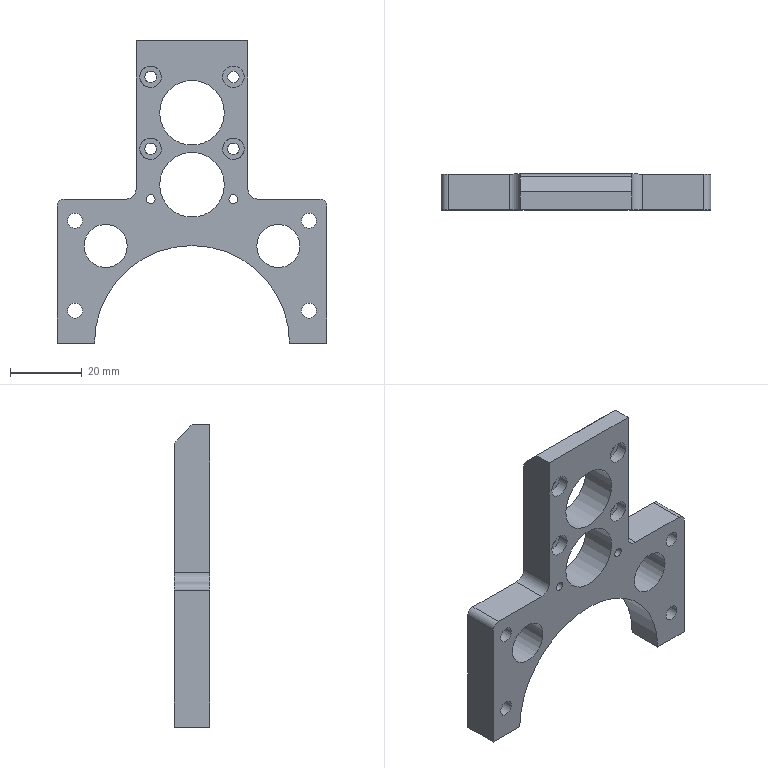Part | NX | 1 solid | 40 faces | box 75 x 10 x 84 mm | volume 23164 mm3 | cylinder 24 | plane 16 | commonest cylinder face diameters 6 x7 3.2 x4 4.2 x4 2.5 x2 4 x2 12 x2
STEP:
#1=CARTESIAN_POINT('',(-15.5,-5.,42.));
#2=VERTEX_POINT('',#1);
#3=CARTESIAN_POINT('',(-15.5,0.,42.));
#4=VERTEX_POINT('',#3);
#5=CARTESIAN_POINT('',(-15.5,-5.,42.));
#6=DIRECTION('',(0.,1.,0.));
#7=VECTOR('',#6,1000.);
#8=LINE('',#5,#7);
#9=EDGE_CURVE('',#2,#4,#8,.T.);
#10=ORIENTED_EDGE('',*,*,#9,.F.);
#11=CARTESIAN_POINT('',(15.5,-5.,42.));
#12=VERTEX_POINT('',#11);
#13=CARTESIAN_POINT('',(-15.5,-5.,42.));
#14=DIRECTION('',(1.,0.,0.));
#15=VECTOR('',#14,1000.);
#16=LINE('',#13,#15);
#17=EDGE_CURVE('',#2,#12,#16,.T.);
#18=ORIENTED_EDGE('',*,*,#17,.T.);
#19=CARTESIAN_POINT('',(15.5,0.,42.));
#20=VERTEX_POINT('',#19);
#21=CARTESIAN_POINT('',(15.5,-5.,42.));
#22=DIRECTION('',(0.,1.,0.));
#23=VECTOR('',#22,1000.);
#24=LINE('',#21,#23);
#25=EDGE_CURVE('',#12,#20,#24,.T.);
#26=ORIENTED_EDGE('',*,*,#25,.T.);
#27=CARTESIAN_POINT('',(-15.5,0.,42.));
#28=DIRECTION('',(1.,0.,0.));
#29=VECTOR('',#28,1000.);
#30=LINE('',#27,#29);
#31=EDGE_CURVE('',#4,#20,#30,.T.);
#32=ORIENTED_EDGE('',*,*,#31,.F.);
#33=EDGE_LOOP('',(#10,#18,#26,#32));
#34=FACE_BOUND('',#33,.T.);
#35=CARTESIAN_POINT('',(-37.5,-5.,42.));
#36=DIRECTION('',(0.,0.,1.));
#37=DIRECTION('',(1.,0.,0.));
#38=AXIS2_PLACEMENT_3D('',#35,#36,#37);
#39=PLANE('',#38);
#40=ADVANCED_FACE('',(#34),#39,.T.);
#41=CARTESIAN_POINT('',(-15.5,4.121,37.879));
#42=VERTEX_POINT('',#41);
#43=CARTESIAN_POINT('',(-15.5,0.,42.));
#44=DIRECTION('',(0.,0.7071,-0.7071));
#45=VECTOR('',#44,1000.);
#46=LINE('',#43,#45);
#47=EDGE_CURVE('',#4,#42,#46,.T.);
#48=ORIENTED_EDGE('',*,*,#47,.F.);
#49=ORIENTED_EDGE('',*,*,#31,.T.);
#50=CARTESIAN_POINT('',(15.5,4.121,37.879));
#51=VERTEX_POINT('',#50);
#52=CARTESIAN_POINT('',(15.5,4.121,37.879));
#53=DIRECTION('',(0.,-0.7071,0.7071));
#54=VECTOR('',#53,1000.);
#55=LINE('',#52,#54);
#56=EDGE_CURVE('',#51,#20,#55,.T.);
#57=ORIENTED_EDGE('',*,*,#56,.F.);
#58=CARTESIAN_POINT('',(-15.5,4.121,37.879));
#59=DIRECTION('',(1.,0.,0.));
#60=VECTOR('',#59,1000.);
#61=LINE('',#58,#60);
#62=EDGE_CURVE('',#42,#51,#61,.T.);
#63=ORIENTED_EDGE('',*,*,#62,.F.);
#64=EDGE_LOOP('',(#48,#49,#57,#63));
#65=FACE_BOUND('',#64,.T.);
#66=CARTESIAN_POINT('',(0.,2.5,39.5));
#67=DIRECTION('',(0.,0.7071,0.7071));
#68=DIRECTION('',(0.,-0.7071,0.7071));
#69=AXIS2_PLACEMENT_3D('',#66,#67,#68);
#70=PLANE('',#69);
#71=ADVANCED_FACE('',(#65),#70,.T.);
#72=CARTESIAN_POINT('',(-15.5,5.,35.757));
#73=VERTEX_POINT('',#72);
#74=CARTESIAN_POINT('',(-15.5,5.,1.));
#75=VERTEX_POINT('',#74);
#76=CARTESIAN_POINT('',(-15.5,5.,35.757));
#77=DIRECTION('',(0.,0.,-1.));
#78=VECTOR('',#77,1000.);
#79=LINE('',#76,#78);
#80=EDGE_CURVE('',#73,#75,#79,.T.);
#81=ORIENTED_EDGE('',*,*,#80,.T.);
#82=CARTESIAN_POINT('',(-15.5,-5.,1.));
#83=VERTEX_POINT('',#82);
#84=CARTESIAN_POINT('',(-15.5,5.,1.));
#85=DIRECTION('',(0.,-1.,0.));
#86=VECTOR('',#85,1000.);
#87=LINE('',#84,#86);
#88=EDGE_CURVE('',#75,#83,#87,.T.);
#89=ORIENTED_EDGE('',*,*,#88,.T.);
#90=CARTESIAN_POINT('',(-15.5,-5.,42.));
#91=DIRECTION('',(0.,0.,-1.));
#92=VECTOR('',#91,1000.);
#93=LINE('',#90,#92);
#94=EDGE_CURVE('',#2,#83,#93,.T.);
#95=ORIENTED_EDGE('',*,*,#94,.F.);
#96=ORIENTED_EDGE('',*,*,#9,.T.);
#97=ORIENTED_EDGE('',*,*,#47,.T.);
#98=CARTESIAN_POINT('',(-15.5,2.,35.757));
#99=DIRECTION('',(-1.,0.,0.));
#100=DIRECTION('',(0.,0.7071,0.7071));
#101=AXIS2_PLACEMENT_3D('',#98,#99,#100);
#102=CIRCLE('',#101,3.);
#103=EDGE_CURVE('',#42,#73,#102,.T.);
#104=ORIENTED_EDGE('',*,*,#103,.T.);
#105=EDGE_LOOP('',(#81,#89,#95,#96,#97,#104));
#106=FACE_BOUND('',#105,.T.);
#107=CARTESIAN_POINT('',(-15.5,5.,42.));
#108=DIRECTION('',(1.,0.,0.));
#109=DIRECTION('',(0.,0.,-1.));
#110=AXIS2_PLACEMENT_3D('',#107,#108,#109);
#111=PLANE('',#110);
#112=ADVANCED_FACE('',(#106),#111,.F.);
#113=CARTESIAN_POINT('',(-18.5,-5.,-2.));
#114=VERTEX_POINT('',#113);
#115=CARTESIAN_POINT('',(-18.5,-5.,1.));
#116=DIRECTION('',(0.,1.,0.));
#117=DIRECTION('',(1.,0.,0.));
#118=AXIS2_PLACEMENT_3D('',#115,#116,#117);
#119=CIRCLE('',#118,3.);
#120=EDGE_CURVE('',#83,#114,#119,.T.);
#121=ORIENTED_EDGE('',*,*,#120,.F.);
#122=ORIENTED_EDGE('',*,*,#88,.F.);
#123=CARTESIAN_POINT('',(-18.5,5.,-2.));
#124=VERTEX_POINT('',#123);
#125=CARTESIAN_POINT('',(-18.5,5.,1.));
#126=DIRECTION('',(0.,-1.,0.));
#127=DIRECTION('',(0.,0.,-1.));
#128=AXIS2_PLACEMENT_3D('',#125,#126,#127);
#129=CIRCLE('',#128,3.);
#130=EDGE_CURVE('',#124,#75,#129,.T.);
#131=ORIENTED_EDGE('',*,*,#130,.F.);
#132=CARTESIAN_POINT('',(-18.5,18.036,-2.));
#133=DIRECTION('',(0.,-1.,0.));
#134=VECTOR('',#133,1000.);
#135=LINE('',#132,#134);
#136=EDGE_CURVE('',#124,#114,#135,.T.);
#137=ORIENTED_EDGE('',*,*,#136,.T.);
#138=EDGE_LOOP('',(#121,#122,#131,#137));
#139=FACE_BOUND('',#138,.T.);
#140=CARTESIAN_POINT('',(-18.5,18.036,1.));
#141=DIRECTION('',(0.,-1.,0.));
#142=DIRECTION('',(0.,0.,-1.));
#143=AXIS2_PLACEMENT_3D('',#140,#141,#142);
#144=CYLINDRICAL_SURFACE('',#143,3.);
#145=ADVANCED_FACE('',(#139),#144,.F.);
#146=CARTESIAN_POINT('',(-35.5,-5.,-2.));
#147=VERTEX_POINT('',#146);
#148=CARTESIAN_POINT('',(37.5,-5.,-2.));
#149=DIRECTION('',(1.,0.,0.));
#150=VECTOR('',#149,1000.);
#151=LINE('',#148,#150);
#152=EDGE_CURVE('',#147,#114,#151,.T.);
#153=ORIENTED_EDGE('',*,*,#152,.T.);
#154=ORIENTED_EDGE('',*,*,#136,.F.);
#155=CARTESIAN_POINT('',(-35.5,5.,-2.));
#156=VERTEX_POINT('',#155);
#157=CARTESIAN_POINT('',(0.,5.,-2.));
#158=DIRECTION('',(1.,0.,0.));
#159=VECTOR('',#158,1000.);
#160=LINE('',#157,#159);
#161=EDGE_CURVE('',#156,#124,#160,.T.);
#162=ORIENTED_EDGE('',*,*,#161,.F.);
#163=CARTESIAN_POINT('',(-35.5,-18.036,-2.));
#164=DIRECTION('',(0.,1.,0.));
#165=VECTOR('',#164,1000.);
#166=LINE('',#163,#165);
#167=EDGE_CURVE('',#147,#156,#166,.T.);
#168=ORIENTED_EDGE('',*,*,#167,.F.);
#169=EDGE_LOOP('',(#153,#154,#162,#168));
#170=FACE_BOUND('',#169,.T.);
#171=CARTESIAN_POINT('',(37.5,5.,-2.));
#172=DIRECTION('',(0.,0.,-1.));
#173=DIRECTION('',(-1.,0.,0.));
#174=AXIS2_PLACEMENT_3D('',#171,#172,#173);
#175=PLANE('',#174);
#176=ADVANCED_FACE('',(#170),#175,.F.);
#177=CARTESIAN_POINT('',(-37.5,-5.,-4.));
#178=VERTEX_POINT('',#177);
#179=CARTESIAN_POINT('',(-37.5,5.,-4.));
#180=VERTEX_POINT('',#179);
#181=CARTESIAN_POINT('',(-37.5,-5.,-4.));
#182=DIRECTION('',(0.,1.,0.));
#183=VECTOR('',#182,1000.);
#184=LINE('',#181,#183);
#185=EDGE_CURVE('',#178,#180,#184,.T.);
#186=ORIENTED_EDGE('',*,*,#185,.F.);
#187=CARTESIAN_POINT('',(-35.5,-5.,-4.));
#188=DIRECTION('',(0.,-1.,0.));
#189=DIRECTION('',(0.,0.,1.));
#190=AXIS2_PLACEMENT_3D('',#187,#188,#189);
#191=CIRCLE('',#190,2.);
#192=EDGE_CURVE('',#147,#178,#191,.T.);
#193=ORIENTED_EDGE('',*,*,#192,.F.);
#194=ORIENTED_EDGE('',*,*,#167,.T.);
#195=CARTESIAN_POINT('',(-35.5,5.,-4.));
#196=DIRECTION('',(0.,1.,0.));
#197=DIRECTION('',(-1.,0.,0.));
#198=AXIS2_PLACEMENT_3D('',#195,#196,#197);
#199=CIRCLE('',#198,2.);
#200=EDGE_CURVE('',#180,#156,#199,.T.);
#201=ORIENTED_EDGE('',*,*,#200,.F.);
#202=EDGE_LOOP('',(#186,#193,#194,#201));
#203=FACE_BOUND('',#202,.T.);
#204=CARTESIAN_POINT('',(-35.5,-18.036,-4.));
#205=DIRECTION('',(0.,1.,0.));
#206=DIRECTION('',(-1.,0.,0.));
#207=AXIS2_PLACEMENT_3D('',#204,#205,#206);
#208=CYLINDRICAL_SURFACE('',#207,2.);
#209=ADVANCED_FACE('',(#203),#208,.T.);
#210=CARTESIAN_POINT('',(-37.5,5.,-42.));
#211=VERTEX_POINT('',#210);
#212=CARTESIAN_POINT('',(-37.5,5.,-42.));
#213=DIRECTION('',(0.,0.,1.));
#214=VECTOR('',#213,1000.);
#215=LINE('',#212,#214);
#216=EDGE_CURVE('',#211,#180,#215,.T.);
#217=ORIENTED_EDGE('',*,*,#216,.F.);
#218=CARTESIAN_POINT('',(-37.5,-5.,-42.));
#219=VERTEX_POINT('',#218);
#220=CARTESIAN_POINT('',(-37.5,-5.,-42.));
#221=DIRECTION('',(0.,1.,0.));
#222=VECTOR('',#221,1000.);
#223=LINE('',#220,#222);
#224=EDGE_CURVE('',#219,#211,#223,.T.);
#225=ORIENTED_EDGE('',*,*,#224,.F.);
#226=CARTESIAN_POINT('',(-37.5,-5.,-42.));
#227=DIRECTION('',(0.,0.,1.));
#228=VECTOR('',#227,1000.);
#229=LINE('',#226,#228);
#230=EDGE_CURVE('',#219,#178,#229,.T.);
#231=ORIENTED_EDGE('',*,*,#230,.T.);
#232=ORIENTED_EDGE('',*,*,#185,.T.);
#233=EDGE_LOOP('',(#217,#225,#231,#232));
#234=FACE_BOUND('',#233,.T.);
#235=CARTESIAN_POINT('',(-37.5,-5.,-42.));
#236=DIRECTION('',(-1.,0.,0.));
#237=DIRECTION('',(0.,0.,1.));
#238=AXIS2_PLACEMENT_3D('',#235,#236,#237);
#239=PLANE('',#238);
#240=ADVANCED_FACE('',(#234),#239,.T.);
#241=CARTESIAN_POINT('',(-27.1,-5.,-42.));
#242=VERTEX_POINT('',#241);
#243=CARTESIAN_POINT('',(-27.1,5.,-42.));
#244=VERTEX_POINT('',#243);
#245=CARTESIAN_POINT('',(-27.1,-5.,-42.));
#246=DIRECTION('',(0.,1.,0.));
#247=VECTOR('',#246,1000.);
#248=LINE('',#245,#247);
#249=EDGE_CURVE('',#242,#244,#248,.T.);
#250=ORIENTED_EDGE('',*,*,#249,.T.);
#251=CARTESIAN_POINT('',(27.1,5.,-42.));
#252=VERTEX_POINT('',#251);
#253=CARTESIAN_POINT('',(0.,5.,-42.));
#254=DIRECTION('',(0.,1.,0.));
#255=DIRECTION('',(-1.,0.,0.));
#256=AXIS2_PLACEMENT_3D('',#253,#254,#255);
#257=CIRCLE('',#256,27.1);
#258=EDGE_CURVE('',#244,#252,#257,.T.);
#259=ORIENTED_EDGE('',*,*,#258,.T.);
#260=CARTESIAN_POINT('',(27.1,-5.,-42.));
#261=VERTEX_POINT('',#260);
#262=CARTESIAN_POINT('',(27.1,-5.,-42.));
#263=DIRECTION('',(0.,1.,0.));
#264=VECTOR('',#263,1000.);
#265=LINE('',#262,#264);
#266=EDGE_CURVE('',#261,#252,#265,.T.);
#267=ORIENTED_EDGE('',*,*,#266,.F.);
#268=CARTESIAN_POINT('',(0.,-5.,-42.));
#269=DIRECTION('',(0.,1.,0.));
#270=DIRECTION('',(-1.,0.,0.));
#271=AXIS2_PLACEMENT_3D('',#268,#269,#270);
#272=CIRCLE('',#271,27.1);
#273=EDGE_CURVE('',#242,#261,#272,.T.);
#274=ORIENTED_EDGE('',*,*,#273,.F.);
#275=EDGE_LOOP('',(#250,#259,#267,#274));
#276=FACE_BOUND('',#275,.T.);
#277=CARTESIAN_POINT('',(0.,5.,-42.));
#278=DIRECTION('',(0.,1.,0.));
#279=DIRECTION('',(1.,0.,0.));
#280=AXIS2_PLACEMENT_3D('',#277,#278,#279);
#281=CYLINDRICAL_SURFACE('',#280,27.1);
#282=ADVANCED_FACE('',(#276),#281,.F.);
#283=ORIENTED_EDGE('',*,*,#224,.T.);
#284=CARTESIAN_POINT('',(-27.1,5.,-42.));
#285=DIRECTION('',(-1.,0.,0.));
#286=VECTOR('',#285,1000.);
#287=LINE('',#284,#286);
#288=EDGE_CURVE('',#244,#211,#287,.T.);
#289=ORIENTED_EDGE('',*,*,#288,.F.);
#290=ORIENTED_EDGE('',*,*,#249,.F.);
#291=CARTESIAN_POINT('',(-27.1,-5.,-42.));
#292=DIRECTION('',(-1.,0.,0.));
#293=VECTOR('',#292,1000.);
#294=LINE('',#291,#293);
#295=EDGE_CURVE('',#242,#219,#294,.T.);
#296=ORIENTED_EDGE('',*,*,#295,.T.);
#297=EDGE_LOOP('',(#283,#289,#290,#296));
#298=FACE_BOUND('',#297,.T.);
#299=CARTESIAN_POINT('',(37.5,-5.,-42.));
#300=DIRECTION('',(0.,0.,-1.));
#301=DIRECTION('',(-1.,0.,0.));
#302=AXIS2_PLACEMENT_3D('',#299,#300,#301);
#303=PLANE('',#302);
#304=ADVANCED_FACE('',(#298),#303,.T.);
#305=ORIENTED_EDGE('',*,*,#266,.T.);
#306=CARTESIAN_POINT('',(37.5,5.,-42.));
#307=VERTEX_POINT('',#306);
#308=CARTESIAN_POINT('',(37.5,5.,-42.));
#309=DIRECTION('',(-1.,0.,0.));
#310=VECTOR('',#309,1000.);
#311=LINE('',#308,#310);
#312=EDGE_CURVE('',#307,#252,#311,.T.);
#313=ORIENTED_EDGE('',*,*,#312,.F.);
#314=CARTESIAN_POINT('',(37.5,-5.,-42.));
#315=VERTEX_POINT('',#314);
#316=CARTESIAN_POINT('',(37.5,-5.,-42.));
#317=DIRECTION('',(0.,1.,0.));
#318=VECTOR('',#317,1000.);
#319=LINE('',#316,#318);
#320=EDGE_CURVE('',#315,#307,#319,.T.);
#321=ORIENTED_EDGE('',*,*,#320,.F.);
#322=CARTESIAN_POINT('',(37.5,-5.,-42.));
#323=DIRECTION('',(-1.,0.,0.));
#324=VECTOR('',#323,1000.);
#325=LINE('',#322,#324);
#326=EDGE_CURVE('',#315,#261,#325,.T.);
#327=ORIENTED_EDGE('',*,*,#326,.T.);
#328=EDGE_LOOP('',(#305,#313,#321,#327));
#329=FACE_BOUND('',#328,.T.);
#330=CARTESIAN_POINT('',(37.5,-5.,-42.));
#331=DIRECTION('',(0.,0.,-1.));
#332=DIRECTION('',(-1.,0.,0.));
#333=AXIS2_PLACEMENT_3D('',#330,#331,#332);
#334=PLANE('',#333);
#335=ADVANCED_FACE('',(#329),#334,.T.);
#336=CARTESIAN_POINT('',(37.5,-5.,-4.));
#337=VERTEX_POINT('',#336);
#338=CARTESIAN_POINT('',(37.5,-5.,-4.));
#339=DIRECTION('',(0.,0.,-1.));
#340=VECTOR('',#339,1000.);
#341=LINE('',#338,#340);
#342=EDGE_CURVE('',#337,#315,#341,.T.);
#343=ORIENTED_EDGE('',*,*,#342,.T.);
#344=ORIENTED_EDGE('',*,*,#320,.T.);
#345=CARTESIAN_POINT('',(37.5,5.,-4.));
#346=VERTEX_POINT('',#345);
#347=CARTESIAN_POINT('',(37.5,5.,-4.));
#348=DIRECTION('',(0.,0.,-1.));
#349=VECTOR('',#348,1000.);
#350=LINE('',#347,#349);
#351=EDGE_CURVE('',#346,#307,#350,.T.);
#352=ORIENTED_EDGE('',*,*,#351,.F.);
#353=CARTESIAN_POINT('',(37.5,5.,-4.));
#354=DIRECTION('',(0.,-1.,0.));
#355=VECTOR('',#354,1000.);
#356=LINE('',#353,#355);
#357=EDGE_CURVE('',#346,#337,#356,.T.);
#358=ORIENTED_EDGE('',*,*,#357,.T.);
#359=EDGE_LOOP('',(#343,#344,#352,#358));
#360=FACE_BOUND('',#359,.T.);
#361=CARTESIAN_POINT('',(37.5,-5.,42.));
#362=DIRECTION('',(1.,0.,0.));
#363=DIRECTION('',(0.,0.,-1.));
#364=AXIS2_PLACEMENT_3D('',#361,#362,#363);
#365=PLANE('',#364);
#366=ADVANCED_FACE('',(#360),#365,.T.);
#367=ORIENTED_EDGE('',*,*,#357,.F.);
#368=CARTESIAN_POINT('',(35.5,5.,-2.));
#369=VERTEX_POINT('',#368);
#370=CARTESIAN_POINT('',(35.5,5.,-4.));
#371=DIRECTION('',(0.,1.,0.));
#372=DIRECTION('',(0.,0.,1.));
#373=AXIS2_PLACEMENT_3D('',#370,#371,#372);
#374=CIRCLE('',#373,2.);
#375=EDGE_CURVE('',#369,#346,#374,.T.);
#376=ORIENTED_EDGE('',*,*,#375,.F.);
#377=CARTESIAN_POINT('',(35.5,-5.,-2.));
#378=VERTEX_POINT('',#377);
#379=CARTESIAN_POINT('',(35.5,5.,-2.));
#380=DIRECTION('',(0.,-1.,0.));
#381=VECTOR('',#380,1000.);
#382=LINE('',#379,#381);
#383=EDGE_CURVE('',#369,#378,#382,.T.);
#384=ORIENTED_EDGE('',*,*,#383,.T.);
#385=CARTESIAN_POINT('',(35.5,-5.,-4.));
#386=DIRECTION('',(0.,-1.,0.));
#387=DIRECTION('',(1.,0.,0.));
#388=AXIS2_PLACEMENT_3D('',#385,#386,#387);
#389=CIRCLE('',#388,2.);
#390=EDGE_CURVE('',#337,#378,#389,.T.);
#391=ORIENTED_EDGE('',*,*,#390,.F.);
#392=EDGE_LOOP('',(#367,#376,#384,#391));
#393=FACE_BOUND('',#392,.T.);
#394=CARTESIAN_POINT('',(35.5,18.036,-4.));
#395=DIRECTION('',(0.,-1.,0.));
#396=DIRECTION('',(1.,0.,0.));
#397=AXIS2_PLACEMENT_3D('',#394,#395,#396);
#398=CYLINDRICAL_SURFACE('',#397,2.);
#399=ADVANCED_FACE('',(#393),#398,.T.);
#400=CARTESIAN_POINT('',(18.5,5.,-2.));
#401=VERTEX_POINT('',#400);
#402=CARTESIAN_POINT('',(35.5,5.,-2.));
#403=DIRECTION('',(-1.,0.,0.));
#404=VECTOR('',#403,1000.);
#405=LINE('',#402,#404);
#406=EDGE_CURVE('',#369,#401,#405,.T.);
#407=ORIENTED_EDGE('',*,*,#406,.T.);
#408=CARTESIAN_POINT('',(18.5,-5.,-2.));
#409=VERTEX_POINT('',#408);
#410=CARTESIAN_POINT('',(18.5,5.,-2.));
#411=DIRECTION('',(0.,-1.,0.));
#412=VECTOR('',#411,1000.);
#413=LINE('',#410,#412);
#414=EDGE_CURVE('',#401,#409,#413,.T.);
#415=ORIENTED_EDGE('',*,*,#414,.T.);
#416=CARTESIAN_POINT('',(35.5,-5.,-2.));
#417=DIRECTION('',(-1.,0.,0.));
#418=VECTOR('',#417,1000.);
#419=LINE('',#416,#418);
#420=EDGE_CURVE('',#378,#409,#419,.T.);
#421=ORIENTED_EDGE('',*,*,#420,.F.);
#422=ORIENTED_EDGE('',*,*,#383,.F.);
#423=EDGE_LOOP('',(#407,#415,#421,#422));
#424=FACE_BOUND('',#423,.T.);
#425=CARTESIAN_POINT('',(37.5,5.,-2.));
#426=DIRECTION('',(0.,0.,-1.));
#427=DIRECTION('',(-1.,0.,0.));
#428=AXIS2_PLACEMENT_3D('',#425,#426,#427);
#429=PLANE('',#428);
#430=ADVANCED_FACE('',(#424),#429,.F.);
#431=CARTESIAN_POINT('',(15.5,-5.,1.));
#432=VERTEX_POINT('',#431);
#433=CARTESIAN_POINT('',(18.5,-5.,1.));
#434=DIRECTION('',(0.,1.,0.));
#435=DIRECTION('',(0.,0.,-1.));
#436=AXIS2_PLACEMENT_3D('',#433,#434,#435);
#437=CIRCLE('',#436,3.);
#438=EDGE_CURVE('',#409,#432,#437,.T.);
#439=ORIENTED_EDGE('',*,*,#438,.F.);
#440=ORIENTED_EDGE('',*,*,#414,.F.);
#441=CARTESIAN_POINT('',(15.5,5.,1.));
#442=VERTEX_POINT('',#441);
#443=CARTESIAN_POINT('',(18.5,5.,1.));
#444=DIRECTION('',(0.,-1.,0.));
#445=DIRECTION('',(-1.,0.,0.));
#446=AXIS2_PLACEMENT_3D('',#443,#444,#445);
#447=CIRCLE('',#446,3.);
#448=EDGE_CURVE('',#442,#401,#447,.T.);
#449=ORIENTED_EDGE('',*,*,#448,.F.);
#450=CARTESIAN_POINT('',(15.5,5.,1.));
#451=DIRECTION('',(0.,-1.,0.));
#452=VECTOR('',#451,1000.);
#453=LINE('',#450,#452);
#454=EDGE_CURVE('',#442,#432,#453,.T.);
#455=ORIENTED_EDGE('',*,*,#454,.T.);
#456=EDGE_LOOP('',(#439,#440,#449,#455));
#457=FACE_BOUND('',#456,.T.);
#458=CARTESIAN_POINT('',(18.5,18.036,1.));
#459=DIRECTION('',(0.,-1.,0.));
#460=DIRECTION('',(-1.,0.,0.));
#461=AXIS2_PLACEMENT_3D('',#458,#459,#460);
#462=CYLINDRICAL_SURFACE('',#461,3.);
#463=ADVANCED_FACE('',(#457),#462,.F.);
#464=ORIENTED_EDGE('',*,*,#56,.T.);
#465=ORIENTED_EDGE('',*,*,#25,.F.);
#466=CARTESIAN_POINT('',(15.5,-5.,42.));
#467=DIRECTION('',(0.,0.,-1.));
#468=VECTOR('',#467,1000.);
#469=LINE('',#466,#468);
#470=EDGE_CURVE('',#12,#432,#469,.T.);
#471=ORIENTED_EDGE('',*,*,#470,.T.);
#472=ORIENTED_EDGE('',*,*,#454,.F.);
#473=CARTESIAN_POINT('',(15.5,5.,35.757));
#474=VERTEX_POINT('',#473);
#475=CARTESIAN_POINT('',(15.5,5.,35.757));
#476=DIRECTION('',(0.,0.,-1.));
#477=VECTOR('',#476,1000.);
#478=LINE('',#475,#477);
#479=EDGE_CURVE('',#474,#442,#478,.T.);
#480=ORIENTED_EDGE('',*,*,#479,.F.);
#481=CARTESIAN_POINT('',(15.5,2.,35.757));
#482=DIRECTION('',(1.,0.,0.));
#483=DIRECTION('',(0.,1.,0.));
#484=AXIS2_PLACEMENT_3D('',#481,#482,#483);
#485=CIRCLE('',#484,3.);
#486=EDGE_CURVE('',#474,#51,#485,.T.);
#487=ORIENTED_EDGE('',*,*,#486,.T.);
#488=EDGE_LOOP('',(#464,#465,#471,#472,#480,#487));
#489=FACE_BOUND('',#488,.T.);
#490=CARTESIAN_POINT('',(15.5,5.,-2.));
#491=DIRECTION('',(-1.,0.,0.));
#492=DIRECTION('',(0.,0.,1.));
#493=AXIS2_PLACEMENT_3D('',#490,#491,#492);
#494=PLANE('',#493);
#495=ADVANCED_FACE('',(#489),#494,.F.);
#496=CARTESIAN_POINT('',(-15.5,5.,35.757));
#497=DIRECTION('',(1.,0.,0.));
#498=VECTOR('',#497,1000.);
#499=LINE('',#496,#498);
#500=EDGE_CURVE('',#73,#474,#499,.T.);
#501=ORIENTED_EDGE('',*,*,#500,.F.);
#502=ORIENTED_EDGE('',*,*,#103,.F.);
#503=ORIENTED_EDGE('',*,*,#62,.T.);
#504=ORIENTED_EDGE('',*,*,#486,.F.);
#505=EDGE_LOOP('',(#501,#502,#503,#504));
#506=FACE_BOUND('',#505,.T.);
#507=CARTESIAN_POINT('',(-135.27,2.,35.757));
#508=DIRECTION('',(1.,0.,0.));
#509=DIRECTION('',(0.,1.,0.));
#510=AXIS2_PLACEMENT_3D('',#507,#508,#509);
#511=CYLINDRICAL_SURFACE('',#510,3.);
#512=ADVANCED_FACE('',(#506),#511,.T.);
#513=CARTESIAN_POINT('',(-18.,5.,-15.));
#514=VERTEX_POINT('',#513);
#515=CARTESIAN_POINT('',(-24.,5.,-15.));
#516=DIRECTION('',(0.,-1.,0.));
#517=DIRECTION('',(1.,0.,0.));
#518=AXIS2_PLACEMENT_3D('',#515,#516,#517);
#519=CIRCLE('',#518,6.);
#520=EDGE_CURVE('',#514,#514,#519,.T.);
#521=ORIENTED_EDGE('',*,*,#520,.F.);
#522=EDGE_LOOP('',(#521));
#523=FACE_BOUND('',#522,.T.);
#524=CARTESIAN_POINT('',(-18.,-5.,-15.));
#525=VERTEX_POINT('',#524);
#526=CARTESIAN_POINT('',(-24.,-5.,-15.));
#527=DIRECTION('',(0.,-1.,0.));
#528=DIRECTION('',(1.,0.,0.));
#529=AXIS2_PLACEMENT_3D('',#526,#527,#528);
#530=CIRCLE('',#529,6.);
#531=EDGE_CURVE('',#525,#525,#530,.T.);
#532=ORIENTED_EDGE('',*,*,#531,.T.);
#533=EDGE_LOOP('',(#532));
#534=FACE_BOUND('',#533,.T.);
#535=CARTESIAN_POINT('',(-24.,-5.,-15.));
#536=DIRECTION('',(0.,-1.,0.));
#537=DIRECTION('',(-1.,0.,0.));
#538=AXIS2_PLACEMENT_3D('',#535,#536,#537);
#539=CYLINDRICAL_SURFACE('',#538,6.);
#540=ADVANCED_FACE('',(#523,#534),#539,.F.);
#541=CARTESIAN_POINT('',(30.,5.,-15.));
#542=VERTEX_POINT('',#541);
#543=CARTESIAN_POINT('',(24.,5.,-15.));
#544=DIRECTION('',(0.,-1.,0.));
#545=DIRECTION('',(1.,0.,0.));
#546=AXIS2_PLACEMENT_3D('',#543,#544,#545);
#547=CIRCLE('',#546,6.);
#548=EDGE_CURVE('',#542,#542,#547,.T.);
#549=ORIENTED_EDGE('',*,*,#548,.F.);
#550=EDGE_LOOP('',(#549));
#551=FACE_BOUND('',#550,.T.);
#552=CARTESIAN_POINT('',(30.,-5.,-15.));
#553=VERTEX_POINT('',#552);
#554=CARTESIAN_POINT('',(24.,-5.,-15.));
#555=DIRECTION('',(0.,-1.,0.));
#556=DIRECTION('',(1.,0.,0.));
#557=AXIS2_PLACEMENT_3D('',#554,#555,#556);
#558=CIRCLE('',#557,6.);
#559=EDGE_CURVE('',#553,#553,#558,.T.);
#560=ORIENTED_EDGE('',*,*,#559,.T.);
#561=EDGE_LOOP('',(#560));
#562=FACE_BOUND('',#561,.T.);
#563=CARTESIAN_POINT('',(24.,-5.,-15.));
#564=DIRECTION('',(0.,-1.,0.));
#565=DIRECTION('',(-1.,0.,0.));
#566=AXIS2_PLACEMENT_3D('',#563,#564,#565);
#567=CYLINDRICAL_SURFACE('',#566,6.);
#568=ADVANCED_FACE('',(#551,#562),#567,.F.);
#569=CARTESIAN_POINT('',(9.,5.,22.));
#570=VERTEX_POINT('',#569);
#571=CARTESIAN_POINT('',(0.,5.,22.));
#572=DIRECTION('',(0.,-1.,0.));
#573=DIRECTION('',(1.,0.,0.));
#574=AXIS2_PLACEMENT_3D('',#571,#572,#573);
#575=CIRCLE('',#574,9.);
#576=EDGE_CURVE('',#570,#570,#575,.T.);
#577=ORIENTED_EDGE('',*,*,#576,.F.);
#578=EDGE_LOOP('',(#577));
#579=FACE_BOUND('',#578,.T.);
#580=CARTESIAN_POINT('',(9.,-5.,22.));
#581=VERTEX_POINT('',#580);
#582=CARTESIAN_POINT('',(0.,-5.,22.));
#583=DIRECTION('',(0.,-1.,0.));
#584=DIRECTION('',(1.,0.,0.));
#585=AXIS2_PLACEMENT_3D('',#582,#583,#584);
#586=CIRCLE('',#585,9.);
#587=EDGE_CURVE('',#581,#581,#586,.T.);
#588=ORIENTED_EDGE('',*,*,#587,.T.);
#589=EDGE_LOOP('',(#588));
#590=FACE_BOUND('',#589,.T.);
#591=CARTESIAN_POINT('',(0.,-5.,22.));
#592=DIRECTION('',(0.,-1.,0.));
#593=DIRECTION('',(-1.,0.,0.));
#594=AXIS2_PLACEMENT_3D('',#591,#592,#593);
#595=CYLINDRICAL_SURFACE('',#594,9.);
#596=ADVANCED_FACE('',(#579,#590),#595,.F.);
#597=CARTESIAN_POINT('',(9.,5.,2.));
#598=VERTEX_POINT('',#597);
#599=CARTESIAN_POINT('',(0.,5.,2.));
#600=DIRECTION('',(0.,-1.,0.));
#601=DIRECTION('',(1.,0.,0.));
#602=AXIS2_PLACEMENT_3D('',#599,#600,#601);
#603=CIRCLE('',#602,9.);
#604=EDGE_CURVE('',#598,#598,#603,.T.);
#605=ORIENTED_EDGE('',*,*,#604,.F.);
#606=EDGE_LOOP('',(#605));
#607=FACE_BOUND('',#606,.T.);
#608=CARTESIAN_POINT('',(9.,-5.,2.));
#609=VERTEX_POINT('',#608);
#610=CARTESIAN_POINT('',(0.,-5.,2.));
#611=DIRECTION('',(0.,-1.,0.));
#612=DIRECTION('',(1.,0.,0.));
#613=AXIS2_PLACEMENT_3D('',#610,#611,#612);
#614=CIRCLE('',#613,9.);
#615=EDGE_CURVE('',#609,#609,#614,.T.);
#616=ORIENTED_EDGE('',*,*,#615,.T.);
#617=EDGE_LOOP('',(#616));
#618=FACE_BOUND('',#617,.T.);
#619=CARTESIAN_POINT('',(0.,-5.,2.));
#620=DIRECTION('',(0.,-1.,0.));
#621=DIRECTION('',(-1.,0.,0.));
#622=AXIS2_PLACEMENT_3D('',#619,#620,#621);
#623=CYLINDRICAL_SURFACE('',#622,9.);
#624=ADVANCED_FACE('',(#607,#618),#623,.F.);
#625=CARTESIAN_POINT('',(12.75,5.,-2.));
#626=VERTEX_POINT('',#625);
#627=CARTESIAN_POINT('',(11.5,5.,-2.));
#628=DIRECTION('',(0.,-1.,0.));
#629=DIRECTION('',(1.,0.,0.));
#630=AXIS2_PLACEMENT_3D('',#627,#628,#629);
#631=CIRCLE('',#630,1.25);
#632=EDGE_CURVE('',#626,#626,#631,.T.);
#633=ORIENTED_EDGE('',*,*,#632,.F.);
#634=EDGE_LOOP('',(#633));
#635=FACE_BOUND('',#634,.T.);
#636=CARTESIAN_POINT('',(12.75,-5.,-2.));
#637=VERTEX_POINT('',#636);
#638=CARTESIAN_POINT('',(11.5,-5.,-2.));
#639=DIRECTION('',(0.,-1.,0.));
#640=DIRECTION('',(1.,0.,0.));
#641=AXIS2_PLACEMENT_3D('',#638,#639,#640);
#642=CIRCLE('',#641,1.25);
#643=EDGE_CURVE('',#637,#637,#642,.T.);
#644=ORIENTED_EDGE('',*,*,#643,.T.);
#645=EDGE_LOOP('',(#644));
#646=FACE_BOUND('',#645,.T.);
#647=CARTESIAN_POINT('',(11.5,-6.55,-2.));
#648=DIRECTION('',(0.,-1.,0.));
#649=DIRECTION('',(-1.,0.,0.));
#650=AXIS2_PLACEMENT_3D('',#647,#648,#649);
#651=CYLINDRICAL_SURFACE('',#650,1.25);
#652=ADVANCED_FACE('',(#635,#646),#651,.F.);
#653=CARTESIAN_POINT('',(-12.75,5.,-2.));
#654=VERTEX_POINT('',#653);
#655=CARTESIAN_POINT('',(-11.5,5.,-2.));
#656=DIRECTION('',(0.,1.,0.));
#657=DIRECTION('',(-1.,0.,0.));
#658=AXIS2_PLACEMENT_3D('',#655,#656,#657);
#659=CIRCLE('',#658,1.25);
#660=EDGE_CURVE('',#654,#654,#659,.T.);
#661=ORIENTED_EDGE('',*,*,#660,.T.);
#662=EDGE_LOOP('',(#661));
#663=FACE_BOUND('',#662,.T.);
#664=CARTESIAN_POINT('',(-12.75,-5.,-2.));
#665=VERTEX_POINT('',#664);
#666=CARTESIAN_POINT('',(-11.5,-5.,-2.));
#667=DIRECTION('',(0.,1.,0.));
#668=DIRECTION('',(-1.,0.,0.));
#669=AXIS2_PLACEMENT_3D('',#666,#667,#668);
#670=CIRCLE('',#669,1.25);
#671=EDGE_CURVE('',#665,#665,#670,.T.);
#672=ORIENTED_EDGE('',*,*,#671,.F.);
#673=EDGE_LOOP('',(#672));
#674=FACE_BOUND('',#673,.T.);
#675=CARTESIAN_POINT('',(-11.5,-6.55,-2.));
#676=DIRECTION('',(0.,1.,0.));
#677=DIRECTION('',(1.,0.,0.));
#678=AXIS2_PLACEMENT_3D('',#675,#676,#677);
#679=CYLINDRICAL_SURFACE('',#678,1.25);
#680=ADVANCED_FACE('',(#663,#674),#679,.F.);
#681=CARTESIAN_POINT('',(-11.5,-2.,9.));
#682=VERTEX_POINT('',#681);
#683=CARTESIAN_POINT('',(-11.5,-2.,12.));
#684=DIRECTION('',(0.,-1.,0.));
#685=DIRECTION('',(0.,0.,-1.));
#686=AXIS2_PLACEMENT_3D('',#683,#684,#685);
#687=CIRCLE('',#686,3.);
#688=EDGE_CURVE('',#682,#682,#687,.T.);
#689=ORIENTED_EDGE('',*,*,#688,.F.);
#690=EDGE_LOOP('',(#689));
#691=FACE_BOUND('',#690,.T.);
#692=CARTESIAN_POINT('',(-14.5,-5.,12.));
#693=VERTEX_POINT('',#692);
#694=CARTESIAN_POINT('',(-11.5,-5.,12.));
#695=DIRECTION('',(0.,1.,0.));
#696=DIRECTION('',(-1.,0.,0.));
#697=AXIS2_PLACEMENT_3D('',#694,#695,#696);
#698=CIRCLE('',#697,3.);
#699=EDGE_CURVE('',#693,#693,#698,.T.);
#700=ORIENTED_EDGE('',*,*,#699,.F.);
#701=EDGE_LOOP('',(#700));
#702=FACE_BOUND('',#701,.T.);
#703=CARTESIAN_POINT('',(-11.5,6.55,12.));
#704=DIRECTION('',(0.,1.,0.));
#705=DIRECTION('',(1.,0.,0.));
#706=AXIS2_PLACEMENT_3D('',#703,#704,#705);
#707=CYLINDRICAL_SURFACE('',#706,3.);
#708=ADVANCED_FACE('',(#691,#702),#707,.F.);
#709=CARTESIAN_POINT('',(-11.5,-2.,10.4));
#710=VERTEX_POINT('',#709);
#711=CARTESIAN_POINT('',(-11.5,-2.,12.));
#712=DIRECTION('',(0.,1.,0.));
#713=DIRECTION('',(0.,0.,-1.));
#714=AXIS2_PLACEMENT_3D('',#711,#712,#713);
#715=CIRCLE('',#714,1.6);
#716=EDGE_CURVE('',#710,#710,#715,.F.);
#717=ORIENTED_EDGE('',*,*,#716,.F.);
#718=EDGE_LOOP('',(#717));
#719=FACE_BOUND('',#718,.T.);
#720=ORIENTED_EDGE('',*,*,#688,.T.);
#721=EDGE_LOOP('',(#720));
#722=FACE_BOUND('',#721,.T.);
#723=CARTESIAN_POINT('',(11.5,-2.,32.));
#724=DIRECTION('',(0.,-1.,0.));
#725=DIRECTION('',(-1.,0.,0.));
#726=AXIS2_PLACEMENT_3D('',#723,#724,#725);
#727=PLANE('',#726);
#728=ADVANCED_FACE('',(#719,#722),#727,.T.);
#729=CARTESIAN_POINT('',(-13.1,5.,12.));
#730=VERTEX_POINT('',#729);
#731=CARTESIAN_POINT('',(-11.5,5.,12.));
#732=DIRECTION('',(0.,1.,0.));
#733=DIRECTION('',(-1.,0.,0.));
#734=AXIS2_PLACEMENT_3D('',#731,#732,#733);
#735=CIRCLE('',#734,1.6);
#736=EDGE_CURVE('',#730,#730,#735,.T.);
#737=ORIENTED_EDGE('',*,*,#736,.T.);
#738=EDGE_LOOP('',(#737));
#739=FACE_BOUND('',#738,.T.);
#740=ORIENTED_EDGE('',*,*,#716,.T.);
#741=EDGE_LOOP('',(#740));
#742=FACE_BOUND('',#741,.T.);
#743=CARTESIAN_POINT('',(-11.5,6.55,12.));
#744=DIRECTION('',(0.,1.,0.));
#745=DIRECTION('',(1.,0.,0.));
#746=AXIS2_PLACEMENT_3D('',#743,#744,#745);
#747=CYLINDRICAL_SURFACE('',#746,1.6);
#748=ADVANCED_FACE('',(#739,#742),#747,.F.);
#749=CARTESIAN_POINT('',(-11.5,-2.,29.));
#750=VERTEX_POINT('',#749);
#751=CARTESIAN_POINT('',(-11.5,-2.,32.));
#752=DIRECTION('',(0.,-1.,0.));
#753=DIRECTION('',(0.,0.,-1.));
#754=AXIS2_PLACEMENT_3D('',#751,#752,#753);
#755=CIRCLE('',#754,3.);
#756=EDGE_CURVE('',#750,#750,#755,.T.);
#757=ORIENTED_EDGE('',*,*,#756,.F.);
#758=EDGE_LOOP('',(#757));
#759=FACE_BOUND('',#758,.T.);
#760=CARTESIAN_POINT('',(-14.5,-5.,32.));
#761=VERTEX_POINT('',#760);
#762=CARTESIAN_POINT('',(-11.5,-5.,32.));
#763=DIRECTION('',(0.,1.,0.));
#764=DIRECTION('',(-1.,0.,0.));
#765=AXIS2_PLACEMENT_3D('',#762,#763,#764);
#766=CIRCLE('',#765,3.);
#767=EDGE_CURVE('',#761,#761,#766,.T.);
#768=ORIENTED_EDGE('',*,*,#767,.F.);
#769=EDGE_LOOP('',(#768));
#770=FACE_BOUND('',#769,.T.);
#771=CARTESIAN_POINT('',(-11.5,6.55,32.));
#772=DIRECTION('',(0.,1.,0.));
#773=DIRECTION('',(1.,0.,0.));
#774=AXIS2_PLACEMENT_3D('',#771,#772,#773);
#775=CYLINDRICAL_SURFACE('',#774,3.);
#776=ADVANCED_FACE('',(#759,#770),#775,.F.);
#777=CARTESIAN_POINT('',(-11.5,-2.,30.4));
#778=VERTEX_POINT('',#777);
#779=CARTESIAN_POINT('',(-11.5,-2.,32.));
#780=DIRECTION('',(0.,1.,0.));
#781=DIRECTION('',(0.,0.,-1.));
#782=AXIS2_PLACEMENT_3D('',#779,#780,#781);
#783=CIRCLE('',#782,1.6);
#784=EDGE_CURVE('',#778,#778,#783,.F.);
#785=ORIENTED_EDGE('',*,*,#784,.F.);
#786=EDGE_LOOP('',(#785));
#787=FACE_BOUND('',#786,.T.);
#788=ORIENTED_EDGE('',*,*,#756,.T.);
#789=EDGE_LOOP('',(#788));
#790=FACE_BOUND('',#789,.T.);
#791=CARTESIAN_POINT('',(11.5,-2.,32.));
#792=DIRECTION('',(0.,-1.,0.));
#793=DIRECTION('',(-1.,0.,0.));
#794=AXIS2_PLACEMENT_3D('',#791,#792,#793);
#795=PLANE('',#794);
#796=ADVANCED_FACE('',(#787,#790),#795,.T.);
#797=CARTESIAN_POINT('',(-13.1,5.,32.));
#798=VERTEX_POINT('',#797);
#799=CARTESIAN_POINT('',(-11.5,5.,32.));
#800=DIRECTION('',(0.,1.,0.));
#801=DIRECTION('',(-1.,0.,0.));
#802=AXIS2_PLACEMENT_3D('',#799,#800,#801);
#803=CIRCLE('',#802,1.6);
#804=EDGE_CURVE('',#798,#798,#803,.T.);
#805=ORIENTED_EDGE('',*,*,#804,.T.);
#806=EDGE_LOOP('',(#805));
#807=FACE_BOUND('',#806,.T.);
#808=ORIENTED_EDGE('',*,*,#784,.T.);
#809=EDGE_LOOP('',(#808));
#810=FACE_BOUND('',#809,.T.);
#811=CARTESIAN_POINT('',(-11.5,6.55,32.));
#812=DIRECTION('',(0.,1.,0.));
#813=DIRECTION('',(1.,0.,0.));
#814=AXIS2_PLACEMENT_3D('',#811,#812,#813);
#815=CYLINDRICAL_SURFACE('',#814,1.6);
#816=ADVANCED_FACE('',(#807,#810),#815,.F.);
#817=CARTESIAN_POINT('',(14.5,-5.,12.));
#818=VERTEX_POINT('',#817);
#819=CARTESIAN_POINT('',(11.5,-5.,12.));
#820=DIRECTION('',(0.,-1.,0.));
#821=DIRECTION('',(1.,0.,0.));
#822=AXIS2_PLACEMENT_3D('',#819,#820,#821);
#823=CIRCLE('',#822,3.);
#824=EDGE_CURVE('',#818,#818,#823,.T.);
#825=ORIENTED_EDGE('',*,*,#824,.T.);
#826=EDGE_LOOP('',(#825));
#827=FACE_BOUND('',#826,.T.);
#828=CARTESIAN_POINT('',(11.5,-2.,9.));
#829=VERTEX_POINT('',#828);
#830=CARTESIAN_POINT('',(11.5,-2.,12.));
#831=DIRECTION('',(0.,1.,0.));
#832=DIRECTION('',(0.,0.,-1.));
#833=AXIS2_PLACEMENT_3D('',#830,#831,#832);
#834=CIRCLE('',#833,3.);
#835=EDGE_CURVE('',#829,#829,#834,.T.);
#836=ORIENTED_EDGE('',*,*,#835,.T.);
#837=EDGE_LOOP('',(#836));
#838=FACE_BOUND('',#837,.T.);
#839=CARTESIAN_POINT('',(11.5,6.55,12.));
#840=DIRECTION('',(0.,-1.,0.));
#841=DIRECTION('',(-1.,0.,0.));
#842=AXIS2_PLACEMENT_3D('',#839,#840,#841);
#843=CYLINDRICAL_SURFACE('',#842,3.);
#844=ADVANCED_FACE('',(#827,#838),#843,.F.);
#845=CARTESIAN_POINT('',(11.5,-2.,10.4));
#846=VERTEX_POINT('',#845);
#847=CARTESIAN_POINT('',(11.5,-2.,12.));
#848=DIRECTION('',(0.,-1.,0.));
#849=DIRECTION('',(0.,0.,-1.));
#850=AXIS2_PLACEMENT_3D('',#847,#848,#849);
#851=CIRCLE('',#850,1.6);
#852=EDGE_CURVE('',#846,#846,#851,.F.);
#853=ORIENTED_EDGE('',*,*,#852,.T.);
#854=EDGE_LOOP('',(#853));
#855=FACE_BOUND('',#854,.T.);
#856=ORIENTED_EDGE('',*,*,#835,.F.);
#857=EDGE_LOOP('',(#856));
#858=FACE_BOUND('',#857,.T.);
#859=CARTESIAN_POINT('',(11.5,-2.,32.));
#860=DIRECTION('',(0.,-1.,0.));
#861=DIRECTION('',(-1.,0.,0.));
#862=AXIS2_PLACEMENT_3D('',#859,#860,#861);
#863=PLANE('',#862);
#864=ADVANCED_FACE('',(#855,#858),#863,.T.);
#865=ORIENTED_EDGE('',*,*,#852,.F.);
#866=EDGE_LOOP('',(#865));
#867=FACE_BOUND('',#866,.T.);
#868=CARTESIAN_POINT('',(13.1,5.,12.));
#869=VERTEX_POINT('',#868);
#870=CARTESIAN_POINT('',(11.5,5.,12.));
#871=DIRECTION('',(0.,-1.,0.));
#872=DIRECTION('',(1.,0.,0.));
#873=AXIS2_PLACEMENT_3D('',#870,#871,#872);
#874=CIRCLE('',#873,1.6);
#875=EDGE_CURVE('',#869,#869,#874,.T.);
#876=ORIENTED_EDGE('',*,*,#875,.F.);
#877=EDGE_LOOP('',(#876));
#878=FACE_BOUND('',#877,.T.);
#879=CARTESIAN_POINT('',(11.5,6.55,12.));
#880=DIRECTION('',(0.,-1.,0.));
#881=DIRECTION('',(-1.,0.,0.));
#882=AXIS2_PLACEMENT_3D('',#879,#880,#881);
#883=CYLINDRICAL_SURFACE('',#882,1.6);
#884=ADVANCED_FACE('',(#867,#878),#883,.F.);
#885=CARTESIAN_POINT('',(14.5,-5.,32.));
#886=VERTEX_POINT('',#885);
#887=CARTESIAN_POINT('',(11.5,-5.,32.));
#888=DIRECTION('',(0.,-1.,0.));
#889=DIRECTION('',(1.,0.,0.));
#890=AXIS2_PLACEMENT_3D('',#887,#888,#889);
#891=CIRCLE('',#890,3.);
#892=EDGE_CURVE('',#886,#886,#891,.T.);
#893=ORIENTED_EDGE('',*,*,#892,.T.);
#894=EDGE_LOOP('',(#893));
#895=FACE_BOUND('',#894,.T.);
#896=CARTESIAN_POINT('',(8.5,-2.,32.));
#897=VERTEX_POINT('',#896);
#898=CARTESIAN_POINT('',(11.5,-2.,32.));
#899=DIRECTION('',(0.,1.,0.));
#900=DIRECTION('',(-1.,0.,0.));
#901=AXIS2_PLACEMENT_3D('',#898,#899,#900);
#902=CIRCLE('',#901,3.);
#903=EDGE_CURVE('',#897,#897,#902,.T.);
#904=ORIENTED_EDGE('',*,*,#903,.T.);
#905=EDGE_LOOP('',(#904));
#906=FACE_BOUND('',#905,.T.);
#907=CARTESIAN_POINT('',(11.5,6.55,32.));
#908=DIRECTION('',(0.,-1.,0.));
#909=DIRECTION('',(-1.,0.,0.));
#910=AXIS2_PLACEMENT_3D('',#907,#908,#909);
#911=CYLINDRICAL_SURFACE('',#910,3.);
#912=ADVANCED_FACE('',(#895,#906),#911,.F.);
#913=CARTESIAN_POINT('',(9.9,-2.,32.));
#914=VERTEX_POINT('',#913);
#915=CARTESIAN_POINT('',(11.5,-2.,32.));
#916=DIRECTION('',(0.,-1.,0.));
#917=DIRECTION('',(-1.,0.,0.));
#918=AXIS2_PLACEMENT_3D('',#915,#916,#917);
#919=CIRCLE('',#918,1.6);
#920=EDGE_CURVE('',#914,#914,#919,.F.);
#921=ORIENTED_EDGE('',*,*,#920,.T.);
#922=EDGE_LOOP('',(#921));
#923=FACE_BOUND('',#922,.T.);
#924=ORIENTED_EDGE('',*,*,#903,.F.);
#925=EDGE_LOOP('',(#924));
#926=FACE_BOUND('',#925,.T.);
#927=CARTESIAN_POINT('',(11.5,-2.,32.));
#928=DIRECTION('',(0.,-1.,0.));
#929=DIRECTION('',(-1.,0.,0.));
#930=AXIS2_PLACEMENT_3D('',#927,#928,#929);
#931=PLANE('',#930);
#932=ADVANCED_FACE('',(#923,#926),#931,.T.);
#933=ORIENTED_EDGE('',*,*,#920,.F.);
#934=EDGE_LOOP('',(#933));
#935=FACE_BOUND('',#934,.T.);
#936=CARTESIAN_POINT('',(13.1,5.,32.));
#937=VERTEX_POINT('',#936);
#938=CARTESIAN_POINT('',(11.5,5.,32.));
#939=DIRECTION('',(0.,-1.,0.));
#940=DIRECTION('',(1.,0.,0.));
#941=AXIS2_PLACEMENT_3D('',#938,#939,#940);
#942=CIRCLE('',#941,1.6);
#943=EDGE_CURVE('',#937,#937,#942,.T.);
#944=ORIENTED_EDGE('',*,*,#943,.F.);
#945=EDGE_LOOP('',(#944));
#946=FACE_BOUND('',#945,.T.);
#947=CARTESIAN_POINT('',(11.5,6.55,32.));
#948=DIRECTION('',(0.,-1.,0.));
#949=DIRECTION('',(-1.,0.,0.));
#950=AXIS2_PLACEMENT_3D('',#947,#948,#949);
#951=CYLINDRICAL_SURFACE('',#950,1.6);
#952=ADVANCED_FACE('',(#935,#946),#951,.F.);
#953=CARTESIAN_POINT('',(30.4,-5.,-33.));
#954=VERTEX_POINT('',#953);
#955=CARTESIAN_POINT('',(32.5,-5.,-33.));
#956=DIRECTION('',(0.,1.,0.));
#957=DIRECTION('',(-1.,0.,0.));
#958=AXIS2_PLACEMENT_3D('',#955,#956,#957);
#959=CIRCLE('',#958,2.1);
#960=EDGE_CURVE('',#954,#954,#959,.T.);
#961=ORIENTED_EDGE('',*,*,#960,.F.);
#962=EDGE_LOOP('',(#961));
#963=FACE_BOUND('',#962,.T.);
#964=CARTESIAN_POINT('',(30.4,5.,-33.));
#965=VERTEX_POINT('',#964);
#966=CARTESIAN_POINT('',(32.5,5.,-33.));
#967=DIRECTION('',(0.,1.,0.));
#968=DIRECTION('',(-1.,0.,0.));
#969=AXIS2_PLACEMENT_3D('',#966,#967,#968);
#970=CIRCLE('',#969,2.1);
#971=EDGE_CURVE('',#965,#965,#970,.T.);
#972=ORIENTED_EDGE('',*,*,#971,.T.);
#973=EDGE_LOOP('',(#972));
#974=FACE_BOUND('',#973,.T.);
#975=CARTESIAN_POINT('',(32.5,5.,-33.));
#976=DIRECTION('',(0.,1.,0.));
#977=DIRECTION('',(1.,0.,0.));
#978=AXIS2_PLACEMENT_3D('',#975,#976,#977);
#979=CYLINDRICAL_SURFACE('',#978,2.1);
#980=ADVANCED_FACE('',(#963,#974),#979,.F.);
#981=CARTESIAN_POINT('',(30.4,-5.,-8.));
#982=VERTEX_POINT('',#981);
#983=CARTESIAN_POINT('',(32.5,-5.,-8.));
#984=DIRECTION('',(0.,1.,0.));
#985=DIRECTION('',(-1.,0.,0.));
#986=AXIS2_PLACEMENT_3D('',#983,#984,#985);
#987=CIRCLE('',#986,2.1);
#988=EDGE_CURVE('',#982,#982,#987,.T.);
#989=ORIENTED_EDGE('',*,*,#988,.F.);
#990=EDGE_LOOP('',(#989));
#991=FACE_BOUND('',#990,.T.);
#992=CARTESIAN_POINT('',(30.4,5.,-8.));
#993=VERTEX_POINT('',#992);
#994=CARTESIAN_POINT('',(32.5,5.,-8.));
#995=DIRECTION('',(0.,1.,0.));
#996=DIRECTION('',(-1.,0.,0.));
#997=AXIS2_PLACEMENT_3D('',#994,#995,#996);
#998=CIRCLE('',#997,2.1);
#999=EDGE_CURVE('',#993,#993,#998,.T.);
#1000=ORIENTED_EDGE('',*,*,#999,.T.);
#1001=EDGE_LOOP('',(#1000));
#1002=FACE_BOUND('',#1001,.T.);
#1003=CARTESIAN_POINT('',(32.5,5.,-8.));
#1004=DIRECTION('',(0.,1.,0.));
#1005=DIRECTION('',(1.,0.,0.));
#1006=AXIS2_PLACEMENT_3D('',#1003,#1004,#1005);
#1007=CYLINDRICAL_SURFACE('',#1006,2.1);
#1008=ADVANCED_FACE('',(#991,#1002),#1007,.F.);
#1009=CARTESIAN_POINT('',(-34.6,-5.,-33.));
#1010=VERTEX_POINT('',#1009);
#1011=CARTESIAN_POINT('',(-32.5,-5.,-33.));
#1012=DIRECTION('',(0.,1.,0.));
#1013=DIRECTION('',(-1.,0.,0.));
#1014=AXIS2_PLACEMENT_3D('',#1011,#1012,#1013);
#1015=CIRCLE('',#1014,2.1);
#1016=EDGE_CURVE('',#1010,#1010,#1015,.T.);
#1017=ORIENTED_EDGE('',*,*,#1016,.F.);
#1018=EDGE_LOOP('',(#1017));
#1019=FACE_BOUND('',#1018,.T.);
#1020=CARTESIAN_POINT('',(-34.6,5.,-33.));
#1021=VERTEX_POINT('',#1020);
#1022=CARTESIAN_POINT('',(-32.5,5.,-33.));
#1023=DIRECTION('',(0.,1.,0.));
#1024=DIRECTION('',(-1.,0.,0.));
#1025=AXIS2_PLACEMENT_3D('',#1022,#1023,#1024);
#1026=CIRCLE('',#1025,2.1);
#1027=EDGE_CURVE('',#1021,#1021,#1026,.T.);
#1028=ORIENTED_EDGE('',*,*,#1027,.T.);
#1029=EDGE_LOOP('',(#1028));
#1030=FACE_BOUND('',#1029,.T.);
#1031=CARTESIAN_POINT('',(-32.5,5.,-33.));
#1032=DIRECTION('',(0.,1.,0.));
#1033=DIRECTION('',(1.,0.,0.));
#1034=AXIS2_PLACEMENT_3D('',#1031,#1032,#1033);
#1035=CYLINDRICAL_SURFACE('',#1034,2.1);
#1036=ADVANCED_FACE('',(#1019,#1030),#1035,.F.);
#1037=CARTESIAN_POINT('',(-30.4,5.,-8.));
#1038=VERTEX_POINT('',#1037);
#1039=CARTESIAN_POINT('',(-32.5,5.,-8.));
#1040=DIRECTION('',(0.,1.,0.));
#1041=DIRECTION('',(1.,0.,0.));
#1042=AXIS2_PLACEMENT_3D('',#1039,#1040,#1041);
#1043=CIRCLE('',#1042,2.1);
#1044=EDGE_CURVE('',#1038,#1038,#1043,.T.);
#1045=ORIENTED_EDGE('',*,*,#1044,.F.);
#1046=EDGE_LOOP('',(#1045));
#1047=FACE_BOUND('',#1046,.T.);
#1048=ORIENTED_EDGE('',*,*,#520,.T.);
#1049=EDGE_LOOP('',(#1048));
#1050=FACE_BOUND('',#1049,.T.);
#1051=ORIENTED_EDGE('',*,*,#548,.T.);
#1052=EDGE_LOOP('',(#1051));
#1053=FACE_BOUND('',#1052,.T.);
#1054=ORIENTED_EDGE('',*,*,#576,.T.);
#1055=EDGE_LOOP('',(#1054));
#1056=FACE_BOUND('',#1055,.T.);
#1057=ORIENTED_EDGE('',*,*,#604,.T.);
#1058=EDGE_LOOP('',(#1057));
#1059=FACE_BOUND('',#1058,.T.);
#1060=ORIENTED_EDGE('',*,*,#632,.T.);
#1061=EDGE_LOOP('',(#1060));
#1062=FACE_BOUND('',#1061,.T.);
#1063=ORIENTED_EDGE('',*,*,#660,.F.);
#1064=EDGE_LOOP('',(#1063));
#1065=FACE_BOUND('',#1064,.T.);
#1066=ORIENTED_EDGE('',*,*,#736,.F.);
#1067=EDGE_LOOP('',(#1066));
#1068=FACE_BOUND('',#1067,.T.);
#1069=ORIENTED_EDGE('',*,*,#804,.F.);
#1070=EDGE_LOOP('',(#1069));
#1071=FACE_BOUND('',#1070,.T.);
#1072=ORIENTED_EDGE('',*,*,#875,.T.);
#1073=EDGE_LOOP('',(#1072));
#1074=FACE_BOUND('',#1073,.T.);
#1075=ORIENTED_EDGE('',*,*,#943,.T.);
#1076=EDGE_LOOP('',(#1075));
#1077=FACE_BOUND('',#1076,.T.);
#1078=ORIENTED_EDGE('',*,*,#971,.F.);
#1079=EDGE_LOOP('',(#1078));
#1080=FACE_BOUND('',#1079,.T.);
#1081=ORIENTED_EDGE('',*,*,#999,.F.);
#1082=EDGE_LOOP('',(#1081));
#1083=FACE_BOUND('',#1082,.T.);
#1084=ORIENTED_EDGE('',*,*,#1027,.F.);
#1085=EDGE_LOOP('',(#1084));
#1086=FACE_BOUND('',#1085,.T.);
#1087=ORIENTED_EDGE('',*,*,#479,.T.);
#1088=ORIENTED_EDGE('',*,*,#448,.T.);
#1089=ORIENTED_EDGE('',*,*,#406,.F.);
#1090=ORIENTED_EDGE('',*,*,#375,.T.);
#1091=ORIENTED_EDGE('',*,*,#351,.T.);
#1092=ORIENTED_EDGE('',*,*,#312,.T.);
#1093=ORIENTED_EDGE('',*,*,#258,.F.);
#1094=ORIENTED_EDGE('',*,*,#288,.T.);
#1095=ORIENTED_EDGE('',*,*,#216,.T.);
#1096=ORIENTED_EDGE('',*,*,#200,.T.);
#1097=ORIENTED_EDGE('',*,*,#161,.T.);
#1098=ORIENTED_EDGE('',*,*,#130,.T.);
#1099=ORIENTED_EDGE('',*,*,#80,.F.);
#1100=ORIENTED_EDGE('',*,*,#500,.T.);
#1101=EDGE_LOOP('',(#1087,#1088,#1089,#1090,#1091,#1092,#1093,#1094,#1095,#1096,#1097,#1098,#1099,#1100));
#1102=FACE_BOUND('',#1101,.T.);
#1103=CARTESIAN_POINT('',(0.,5.,0.));
#1104=DIRECTION('',(0.,1.,0.));
#1105=DIRECTION('',(1.,0.,0.));
#1106=AXIS2_PLACEMENT_3D('',#1103,#1104,#1105);
#1107=PLANE('',#1106);
#1108=ADVANCED_FACE('',(#1047,#1050,#1053,#1056,#1059,#1062,#1065,#1068,#1071,#1074,#1077,#1080,#1083,#1086,#1102),#1107,.T.);
#1109=CARTESIAN_POINT('',(-34.6,-5.,-8.));
#1110=VERTEX_POINT('',#1109);
#1111=CARTESIAN_POINT('',(-32.5,-5.,-8.));
#1112=DIRECTION('',(0.,1.,0.));
#1113=DIRECTION('',(-1.,0.,0.));
#1114=AXIS2_PLACEMENT_3D('',#1111,#1112,#1113);
#1115=CIRCLE('',#1114,2.1);
#1116=EDGE_CURVE('',#1110,#1110,#1115,.T.);
#1117=ORIENTED_EDGE('',*,*,#1116,.F.);
#1118=EDGE_LOOP('',(#1117));
#1119=FACE_BOUND('',#1118,.T.);
#1120=ORIENTED_EDGE('',*,*,#1044,.T.);
#1121=EDGE_LOOP('',(#1120));
#1122=FACE_BOUND('',#1121,.T.);
#1123=CARTESIAN_POINT('',(-32.5,5.,-8.));
#1124=DIRECTION('',(0.,1.,0.));
#1125=DIRECTION('',(1.,0.,0.));
#1126=AXIS2_PLACEMENT_3D('',#1123,#1124,#1125);
#1127=CYLINDRICAL_SURFACE('',#1126,2.1);
#1128=ADVANCED_FACE('',(#1119,#1122),#1127,.F.);
#1129=ORIENTED_EDGE('',*,*,#531,.F.);
#1130=EDGE_LOOP('',(#1129));
#1131=FACE_BOUND('',#1130,.T.);
#1132=ORIENTED_EDGE('',*,*,#559,.F.);
#1133=EDGE_LOOP('',(#1132));
#1134=FACE_BOUND('',#1133,.T.);
#1135=ORIENTED_EDGE('',*,*,#587,.F.);
#1136=EDGE_LOOP('',(#1135));
#1137=FACE_BOUND('',#1136,.T.);
#1138=ORIENTED_EDGE('',*,*,#615,.F.);
#1139=EDGE_LOOP('',(#1138));
#1140=FACE_BOUND('',#1139,.T.);
#1141=ORIENTED_EDGE('',*,*,#1116,.T.);
#1142=EDGE_LOOP('',(#1141));
#1143=FACE_BOUND('',#1142,.T.);
#1144=ORIENTED_EDGE('',*,*,#643,.F.);
#1145=EDGE_LOOP('',(#1144));
#1146=FACE_BOUND('',#1145,.T.);
#1147=ORIENTED_EDGE('',*,*,#671,.T.);
#1148=EDGE_LOOP('',(#1147));
#1149=FACE_BOUND('',#1148,.T.);
#1150=ORIENTED_EDGE('',*,*,#699,.T.);
#1151=EDGE_LOOP('',(#1150));
#1152=FACE_BOUND('',#1151,.T.);
#1153=ORIENTED_EDGE('',*,*,#767,.T.);
#1154=EDGE_LOOP('',(#1153));
#1155=FACE_BOUND('',#1154,.T.);
#1156=ORIENTED_EDGE('',*,*,#824,.F.);
#1157=EDGE_LOOP('',(#1156));
#1158=FACE_BOUND('',#1157,.T.);
#1159=ORIENTED_EDGE('',*,*,#892,.F.);
#1160=EDGE_LOOP('',(#1159));
#1161=FACE_BOUND('',#1160,.T.);
#1162=ORIENTED_EDGE('',*,*,#960,.T.);
#1163=EDGE_LOOP('',(#1162));
#1164=FACE_BOUND('',#1163,.T.);
#1165=ORIENTED_EDGE('',*,*,#988,.T.);
#1166=EDGE_LOOP('',(#1165));
#1167=FACE_BOUND('',#1166,.T.);
#1168=ORIENTED_EDGE('',*,*,#1016,.T.);
#1169=EDGE_LOOP('',(#1168));
#1170=FACE_BOUND('',#1169,.T.);
#1171=ORIENTED_EDGE('',*,*,#420,.T.);
#1172=ORIENTED_EDGE('',*,*,#438,.T.);
#1173=ORIENTED_EDGE('',*,*,#470,.F.);
#1174=ORIENTED_EDGE('',*,*,#17,.F.);
#1175=ORIENTED_EDGE('',*,*,#94,.T.);
#1176=ORIENTED_EDGE('',*,*,#120,.T.);
#1177=ORIENTED_EDGE('',*,*,#152,.F.);
#1178=ORIENTED_EDGE('',*,*,#192,.T.);
#1179=ORIENTED_EDGE('',*,*,#230,.F.);
#1180=ORIENTED_EDGE('',*,*,#295,.F.);
#1181=ORIENTED_EDGE('',*,*,#273,.T.);
#1182=ORIENTED_EDGE('',*,*,#326,.F.);
#1183=ORIENTED_EDGE('',*,*,#342,.F.);
#1184=ORIENTED_EDGE('',*,*,#390,.T.);
#1185=EDGE_LOOP('',(#1171,#1172,#1173,#1174,#1175,#1176,#1177,#1178,#1179,#1180,#1181,#1182,#1183,#1184));
#1186=FACE_BOUND('',#1185,.T.);
#1187=CARTESIAN_POINT('',(0.,-5.,0.));
#1188=DIRECTION('',(0.,1.,0.));
#1189=DIRECTION('',(1.,0.,0.));
#1190=AXIS2_PLACEMENT_3D('',#1187,#1188,#1189);
#1191=PLANE('',#1190);
#1192=ADVANCED_FACE('',(#1131,#1134,#1137,#1140,#1143,#1146,#1149,#1152,#1155,#1158,#1161,#1164,#1167,#1170,#1186),#1191,.F.);
#1193=CLOSED_SHELL('',(#40,#71,#112,#145,#176,#209,#240,#282,#304,#335,#366,#399,#430,#463,#495,#512,#540,#568,#596,#624,#652,#680,#708,#728,#748,#776,#796,#816,#844,#864,#884,#912,#932,#952,#980,#1008,#1036,#1108,#1128,#1192));
#1194=MANIFOLD_SOLID_BREP('',#1193);
#1195=(LENGTH_UNIT()NAMED_UNIT(*)SI_UNIT(.MILLI.,.METRE.));
#1196=UNCERTAINTY_MEASURE_WITH_UNIT(LENGTH_MEASURE(0.00001),#1195,'','');
#1197=(NAMED_UNIT(*)PLANE_ANGLE_UNIT()SI_UNIT($,.RADIAN.));
#1198=(NAMED_UNIT(*)SI_UNIT($,.STERADIAN.)SOLID_ANGLE_UNIT());
#1199=(GEOMETRIC_REPRESENTATION_CONTEXT(3)GLOBAL_UNCERTAINTY_ASSIGNED_CONTEXT((#1196))GLOBAL_UNIT_ASSIGNED_CONTEXT((#1195,#1197,#1198))REPRESENTATION_CONTEXT('',''));
#1200=ADVANCED_BREP_SHAPE_REPRESENTATION('',(#1194),#1199);